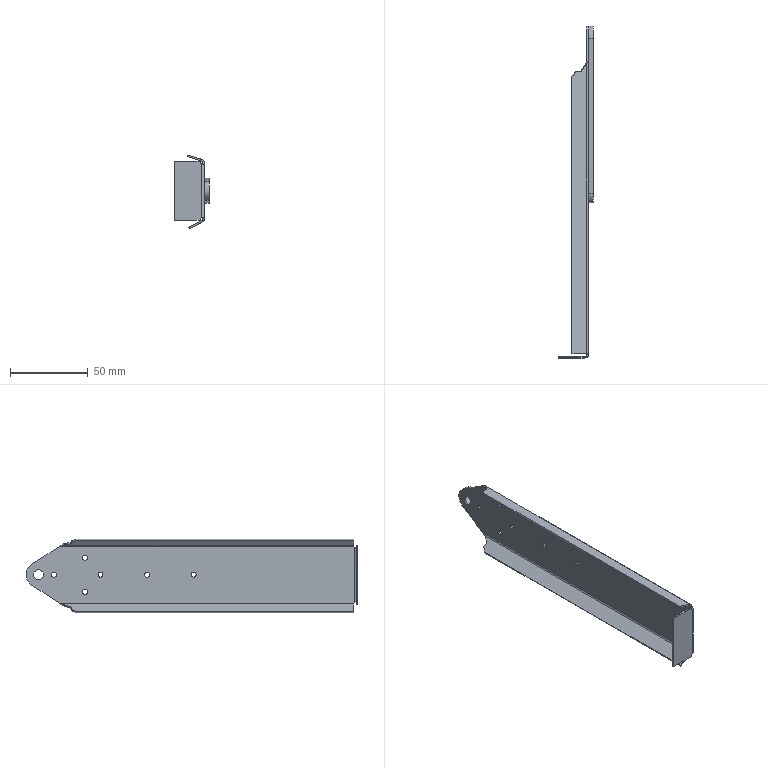Part | SolidWorks | features BaseBody 2 | 2 solids | 74 faces | box 22.422 x 213.912 x 47.633 mm | volume 17053 mm3 | cylinder 41 | plane 27 | spline 6 | commonest cylinder face diameters 3.2 x20 4 x7 6.35 x4 16 x4 2 x3 5 x2